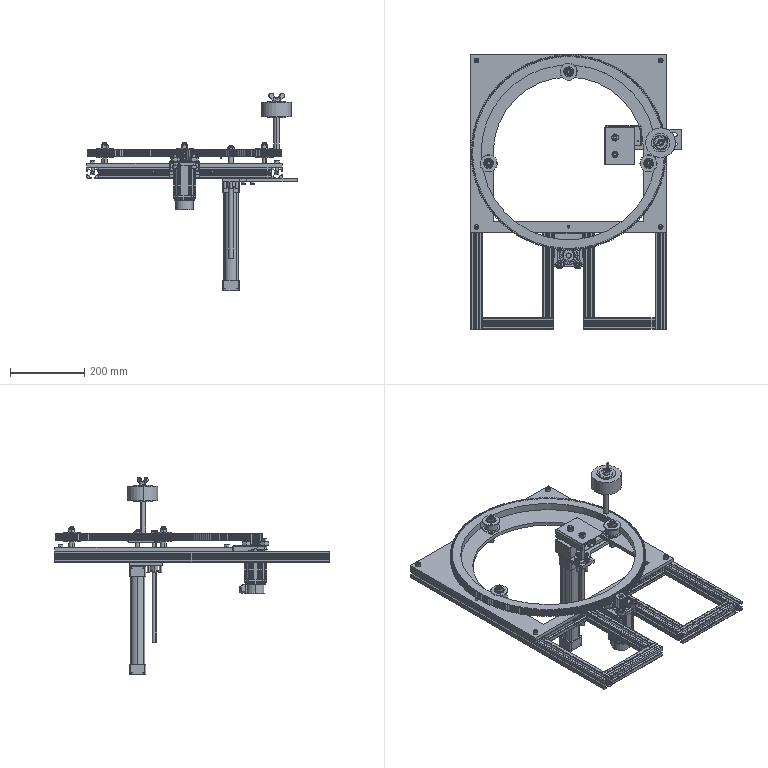Part | SolidWorks | features CompositeCurve 5, ReferencePattern 5, MirrorCompFeat 1 | 161 solids | 6684 faces | volume 4381513 mm3 | cylinder 2506 | plane 2346 | spline 631 | sphere 436 | cone 402 | torus 363 | commonest cylinder face diameters 514.994 x261 524 x260 10 x251 0.4 x216 1.6 x166 17.2 x126